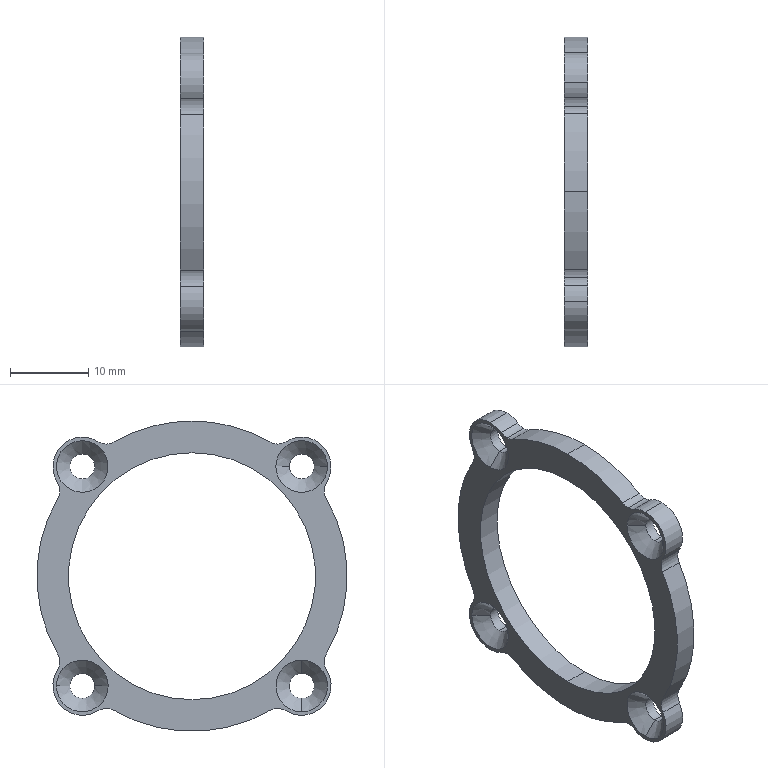Part | SolidWorks | features RefAxis 2, CirPattern 1, Extrusion 1, Fillet 1, RevCut 1 | 1 solid | 41 faces | box 3 x 39.6 x 39.6 mm | volume 1466 mm3 | cylinder 31 | cone 8 | plane 2 | commonest cylinder face diameters 4 x10 3.2 x8 7.5 x6 39.6 x5 31.5 x2
STEP:
#1=CARTESIAN_POINT('',(0.,10.93,16.862));
#2=VERTEX_POINT('',#1);
#3=CARTESIAN_POINT('',(0.,11.998,17.171));
#4=VERTEX_POINT('',#3);
#5=CARTESIAN_POINT('',(0.,10.93,18.862));
#6=DIRECTION('',(1.,0.,0.));
#7=DIRECTION('',(0.,0.,-1.));
#8=AXIS2_PLACEMENT_3D('',#5,#6,#7);
#9=CIRCLE('',#8,2.);
#10=EDGE_CURVE('',#2,#4,#9,.T.);
#11=ORIENTED_EDGE('',*,*,#10,.F.);
#12=CARTESIAN_POINT('',(3.,10.93,16.862));
#13=VERTEX_POINT('',#12);
#14=CARTESIAN_POINT('',(3.,10.93,16.862));
#15=DIRECTION('',(1.,0.,0.));
#16=VECTOR('',#15,1000.);
#17=LINE('',#14,#16);
#18=EDGE_CURVE('',#2,#13,#17,.T.);
#19=ORIENTED_EDGE('',*,*,#18,.T.);
#20=CARTESIAN_POINT('',(3.,11.998,17.171));
#21=VERTEX_POINT('',#20);
#22=CARTESIAN_POINT('',(3.,10.93,18.862));
#23=DIRECTION('',(-1.,0.,0.));
#24=DIRECTION('',(0.,0.,-1.));
#25=AXIS2_PLACEMENT_3D('',#22,#23,#24);
#26=CIRCLE('',#25,2.);
#27=EDGE_CURVE('',#21,#13,#26,.T.);
#28=ORIENTED_EDGE('',*,*,#27,.F.);
#29=CARTESIAN_POINT('',(3.,11.998,17.171));
#30=DIRECTION('',(1.,0.,0.));
#31=VECTOR('',#30,1000.);
#32=LINE('',#29,#31);
#33=EDGE_CURVE('',#4,#21,#32,.T.);
#34=ORIENTED_EDGE('',*,*,#33,.F.);
#35=EDGE_LOOP('',(#11,#19,#28,#34));
#36=FACE_OUTER_BOUND('',#35,.T.);
#37=CARTESIAN_POINT('',(3.,10.93,18.862));
#38=DIRECTION('',(1.,0.,0.));
#39=DIRECTION('',(0.,0.,-1.));
#40=AXIS2_PLACEMENT_3D('',#37,#38,#39);
#41=CYLINDRICAL_SURFACE('',#40,2.);
#42=ADVANCED_FACE('',(#36),#41,.F.);
#43=CARTESIAN_POINT('',(0.,-10.93,16.862));
#44=VERTEX_POINT('',#43);
#45=CARTESIAN_POINT('',(0.,-9.927,17.132));
#46=VERTEX_POINT('',#45);
#47=CARTESIAN_POINT('',(0.,-10.93,18.862));
#48=DIRECTION('',(1.,0.,0.));
#49=DIRECTION('',(0.,0.,-1.));
#50=AXIS2_PLACEMENT_3D('',#47,#48,#49);
#51=CIRCLE('',#50,2.);
#52=EDGE_CURVE('',#44,#46,#51,.T.);
#53=ORIENTED_EDGE('',*,*,#52,.F.);
#54=CARTESIAN_POINT('',(3.,-10.93,16.862));
#55=VERTEX_POINT('',#54);
#56=CARTESIAN_POINT('',(3.,-10.93,16.862));
#57=DIRECTION('',(1.,0.,0.));
#58=VECTOR('',#57,1000.);
#59=LINE('',#56,#58);
#60=EDGE_CURVE('',#44,#55,#59,.T.);
#61=ORIENTED_EDGE('',*,*,#60,.T.);
#62=CARTESIAN_POINT('',(3.,-9.927,17.132));
#63=VERTEX_POINT('',#62);
#64=CARTESIAN_POINT('',(3.,-10.93,18.862));
#65=DIRECTION('',(-1.,0.,0.));
#66=DIRECTION('',(0.,0.,-1.));
#67=AXIS2_PLACEMENT_3D('',#64,#65,#66);
#68=CIRCLE('',#67,2.);
#69=EDGE_CURVE('',#63,#55,#68,.T.);
#70=ORIENTED_EDGE('',*,*,#69,.F.);
#71=CARTESIAN_POINT('',(3.,-9.927,17.132));
#72=DIRECTION('',(1.,0.,0.));
#73=VECTOR('',#72,1000.);
#74=LINE('',#71,#73);
#75=EDGE_CURVE('',#46,#63,#74,.T.);
#76=ORIENTED_EDGE('',*,*,#75,.F.);
#77=EDGE_LOOP('',(#53,#61,#70,#76));
#78=FACE_OUTER_BOUND('',#77,.T.);
#79=CARTESIAN_POINT('',(3.,-10.93,18.862));
#80=DIRECTION('',(1.,0.,0.));
#81=DIRECTION('',(0.,0.,-1.));
#82=AXIS2_PLACEMENT_3D('',#79,#80,#81);
#83=CYLINDRICAL_SURFACE('',#82,2.);
#84=ADVANCED_FACE('',(#78),#83,.F.);
#85=CARTESIAN_POINT('',(1.7,14.001,-12.401));
#86=VERTEX_POINT('',#85);
#87=CARTESIAN_POINT('',(1.7,12.401,-14.001));
#88=VERTEX_POINT('',#87);
#89=CARTESIAN_POINT('',(1.7,14.001,-14.001));
#90=DIRECTION('',(1.,0.,0.));
#91=DIRECTION('',(0.,0.,1.));
#92=AXIS2_PLACEMENT_3D('',#89,#90,#91);
#93=CIRCLE('',#92,1.6);
#94=EDGE_CURVE('',#86,#88,#93,.T.);
#95=ORIENTED_EDGE('',*,*,#94,.T.);
#96=CARTESIAN_POINT('',(0.,10.701,-14.001));
#97=VERTEX_POINT('',#96);
#98=CARTESIAN_POINT('',(3.3,14.001,-14.001));
#99=DIRECTION('',(-0.7071,-0.7071,0.));
#100=VECTOR('',#99,1000.);
#101=LINE('',#98,#100);
#102=EDGE_CURVE('',#88,#97,#101,.T.);
#103=ORIENTED_EDGE('',*,*,#102,.T.);
#104=CARTESIAN_POINT('',(0.,17.301,-14.001));
#105=VERTEX_POINT('',#104);
#106=CARTESIAN_POINT('',(0.,14.001,-14.001));
#107=DIRECTION('',(1.,0.,0.));
#108=DIRECTION('',(0.,-1.,0.));
#109=AXIS2_PLACEMENT_3D('',#106,#107,#108);
#110=CIRCLE('',#109,3.3);
#111=EDGE_CURVE('',#105,#97,#110,.T.);
#112=ORIENTED_EDGE('',*,*,#111,.F.);
#113=CARTESIAN_POINT('',(1.7,15.601,-14.001));
#114=VERTEX_POINT('',#113);
#115=CARTESIAN_POINT('',(3.3,14.001,-14.001));
#116=DIRECTION('',(-0.7071,0.7071,0.));
#117=VECTOR('',#116,1000.);
#118=LINE('',#115,#117);
#119=EDGE_CURVE('',#114,#105,#118,.T.);
#120=ORIENTED_EDGE('',*,*,#119,.F.);
#121=CARTESIAN_POINT('',(1.7,14.001,-14.001));
#122=DIRECTION('',(1.,0.,0.));
#123=DIRECTION('',(0.,0.,1.));
#124=AXIS2_PLACEMENT_3D('',#121,#122,#123);
#125=CIRCLE('',#124,1.6);
#126=EDGE_CURVE('',#114,#86,#125,.T.);
#127=ORIENTED_EDGE('',*,*,#126,.T.);
#128=EDGE_LOOP('',(#95,#103,#112,#120,#127));
#129=FACE_OUTER_BOUND('',#128,.T.);
#130=CARTESIAN_POINT('',(-996.7,14.001,-14.001));
#131=DIRECTION('',(-1.,0.,0.));
#132=DIRECTION('',(0.,1.,0.));
#133=AXIS2_PLACEMENT_3D('',#130,#131,#132);
#134=CONICAL_SURFACE('',#133,1000.,0.7854);
#135=ADVANCED_FACE('',(#129),#134,.F.);
#136=CARTESIAN_POINT('',(1.7,-14.001,-15.601));
#137=VERTEX_POINT('',#136);
#138=CARTESIAN_POINT('',(1.7,-14.001,-12.401));
#139=VERTEX_POINT('',#138);
#140=CARTESIAN_POINT('',(1.7,-14.001,-14.001));
#141=DIRECTION('',(1.,0.,0.));
#142=DIRECTION('',(0.,0.,1.));
#143=AXIS2_PLACEMENT_3D('',#140,#141,#142);
#144=CIRCLE('',#143,1.6);
#145=EDGE_CURVE('',#137,#139,#144,.T.);
#146=ORIENTED_EDGE('',*,*,#145,.T.);
#147=CARTESIAN_POINT('',(0.,-14.001,-10.701));
#148=VERTEX_POINT('',#147);
#149=CARTESIAN_POINT('',(3.3,-14.001,-14.001));
#150=DIRECTION('',(-0.7071,0.,0.7071));
#151=VECTOR('',#150,1000.);
#152=LINE('',#149,#151);
#153=EDGE_CURVE('',#139,#148,#152,.T.);
#154=ORIENTED_EDGE('',*,*,#153,.T.);
#155=CARTESIAN_POINT('',(0.,-14.001,-17.301));
#156=VERTEX_POINT('',#155);
#157=CARTESIAN_POINT('',(0.,-14.001,-14.001));
#158=DIRECTION('',(1.,0.,0.));
#159=DIRECTION('',(0.,0.,1.));
#160=AXIS2_PLACEMENT_3D('',#157,#158,#159);
#161=CIRCLE('',#160,3.3);
#162=EDGE_CURVE('',#156,#148,#161,.T.);
#163=ORIENTED_EDGE('',*,*,#162,.F.);
#164=CARTESIAN_POINT('',(3.3,-14.001,-14.001));
#165=DIRECTION('',(-0.7071,0.,-0.7071));
#166=VECTOR('',#165,1000.);
#167=LINE('',#164,#166);
#168=EDGE_CURVE('',#137,#156,#167,.T.);
#169=ORIENTED_EDGE('',*,*,#168,.F.);
#170=EDGE_LOOP('',(#146,#154,#163,#169));
#171=FACE_OUTER_BOUND('',#170,.T.);
#172=CARTESIAN_POINT('',(-996.7,-14.001,-14.001));
#173=DIRECTION('',(-1.,0.,0.));
#174=DIRECTION('',(0.,0.,-1.));
#175=AXIS2_PLACEMENT_3D('',#172,#173,#174);
#176=CONICAL_SURFACE('',#175,1000.,0.7854);
#177=ADVANCED_FACE('',(#171),#176,.F.);
#178=CARTESIAN_POINT('',(1.7,-14.001,12.401));
#179=VERTEX_POINT('',#178);
#180=CARTESIAN_POINT('',(1.7,-12.401,14.001));
#181=VERTEX_POINT('',#180);
#182=CARTESIAN_POINT('',(1.7,-14.001,14.001));
#183=DIRECTION('',(1.,0.,0.));
#184=DIRECTION('',(0.,0.,1.));
#185=AXIS2_PLACEMENT_3D('',#182,#183,#184);
#186=CIRCLE('',#185,1.6);
#187=EDGE_CURVE('',#179,#181,#186,.T.);
#188=ORIENTED_EDGE('',*,*,#187,.T.);
#189=CARTESIAN_POINT('',(0.,-10.701,14.001));
#190=VERTEX_POINT('',#189);
#191=CARTESIAN_POINT('',(3.3,-14.001,14.001));
#192=DIRECTION('',(-0.7071,0.7071,0.));
#193=VECTOR('',#192,1000.);
#194=LINE('',#191,#193);
#195=EDGE_CURVE('',#181,#190,#194,.T.);
#196=ORIENTED_EDGE('',*,*,#195,.T.);
#197=CARTESIAN_POINT('',(0.,-17.301,14.001));
#198=VERTEX_POINT('',#197);
#199=CARTESIAN_POINT('',(0.,-14.001,14.001));
#200=DIRECTION('',(1.,0.,0.));
#201=DIRECTION('',(0.,1.,0.));
#202=AXIS2_PLACEMENT_3D('',#199,#200,#201);
#203=CIRCLE('',#202,3.3);
#204=EDGE_CURVE('',#198,#190,#203,.T.);
#205=ORIENTED_EDGE('',*,*,#204,.F.);
#206=CARTESIAN_POINT('',(1.7,-15.601,14.001));
#207=VERTEX_POINT('',#206);
#208=CARTESIAN_POINT('',(3.3,-14.001,14.001));
#209=DIRECTION('',(-0.7071,-0.7071,0.));
#210=VECTOR('',#209,1000.);
#211=LINE('',#208,#210);
#212=EDGE_CURVE('',#207,#198,#211,.T.);
#213=ORIENTED_EDGE('',*,*,#212,.F.);
#214=CARTESIAN_POINT('',(1.7,-14.001,14.001));
#215=DIRECTION('',(1.,0.,0.));
#216=DIRECTION('',(0.,0.,1.));
#217=AXIS2_PLACEMENT_3D('',#214,#215,#216);
#218=CIRCLE('',#217,1.6);
#219=EDGE_CURVE('',#207,#179,#218,.T.);
#220=ORIENTED_EDGE('',*,*,#219,.T.);
#221=EDGE_LOOP('',(#188,#196,#205,#213,#220));
#222=FACE_OUTER_BOUND('',#221,.T.);
#223=CARTESIAN_POINT('',(-996.7,-14.001,14.001));
#224=DIRECTION('',(-1.,0.,0.));
#225=DIRECTION('',(0.,-1.,0.));
#226=AXIS2_PLACEMENT_3D('',#223,#224,#225);
#227=CONICAL_SURFACE('',#226,1000.,0.7854);
#228=ADVANCED_FACE('',(#222),#227,.F.);
#229=CARTESIAN_POINT('',(1.7,14.001,15.601));
#230=VERTEX_POINT('',#229);
#231=CARTESIAN_POINT('',(1.7,14.001,12.401));
#232=VERTEX_POINT('',#231);
#233=CARTESIAN_POINT('',(1.7,14.001,14.001));
#234=DIRECTION('',(1.,0.,0.));
#235=DIRECTION('',(0.,0.,1.));
#236=AXIS2_PLACEMENT_3D('',#233,#234,#235);
#237=CIRCLE('',#236,1.6);
#238=EDGE_CURVE('',#230,#232,#237,.T.);
#239=ORIENTED_EDGE('',*,*,#238,.T.);
#240=CARTESIAN_POINT('',(0.,14.001,10.701));
#241=VERTEX_POINT('',#240);
#242=CARTESIAN_POINT('',(3.3,14.001,14.001));
#243=DIRECTION('',(-0.7071,0.,-0.7071));
#244=VECTOR('',#243,1000.);
#245=LINE('',#242,#244);
#246=EDGE_CURVE('',#232,#241,#245,.T.);
#247=ORIENTED_EDGE('',*,*,#246,.T.);
#248=CARTESIAN_POINT('',(0.,14.001,17.301));
#249=VERTEX_POINT('',#248);
#250=CARTESIAN_POINT('',(0.,14.001,14.001));
#251=DIRECTION('',(1.,0.,0.));
#252=DIRECTION('',(0.,0.,-1.));
#253=AXIS2_PLACEMENT_3D('',#250,#251,#252);
#254=CIRCLE('',#253,3.3);
#255=EDGE_CURVE('',#249,#241,#254,.T.);
#256=ORIENTED_EDGE('',*,*,#255,.F.);
#257=CARTESIAN_POINT('',(3.3,14.001,14.001));
#258=DIRECTION('',(-0.7071,0.,0.7071));
#259=VECTOR('',#258,1000.);
#260=LINE('',#257,#259);
#261=EDGE_CURVE('',#230,#249,#260,.T.);
#262=ORIENTED_EDGE('',*,*,#261,.F.);
#263=EDGE_LOOP('',(#239,#247,#256,#262));
#264=FACE_OUTER_BOUND('',#263,.T.);
#265=CARTESIAN_POINT('',(-996.7,14.001,14.001));
#266=DIRECTION('',(-1.,0.,0.));
#267=DIRECTION('',(0.,0.,1.));
#268=AXIS2_PLACEMENT_3D('',#265,#266,#267);
#269=CONICAL_SURFACE('',#268,1000.,0.7854);
#270=ADVANCED_FACE('',(#264),#269,.F.);
#271=CARTESIAN_POINT('',(3.,14.001,-12.401));
#272=VERTEX_POINT('',#271);
#273=CARTESIAN_POINT('',(3.,14.001,-15.601));
#274=VERTEX_POINT('',#273);
#275=CARTESIAN_POINT('',(3.,14.001,-14.001));
#276=DIRECTION('',(1.,0.,0.));
#277=DIRECTION('',(0.,0.,-1.));
#278=AXIS2_PLACEMENT_3D('',#275,#276,#277);
#279=CIRCLE('',#278,1.6);
#280=EDGE_CURVE('',#272,#274,#279,.T.);
#281=ORIENTED_EDGE('',*,*,#280,.T.);
#282=CARTESIAN_POINT('',(1.7,14.001,-15.601));
#283=VERTEX_POINT('',#282);
#284=CARTESIAN_POINT('',(3.,14.001,-15.601));
#285=DIRECTION('',(-1.,0.,0.));
#286=VECTOR('',#285,1000.);
#287=LINE('',#284,#286);
#288=EDGE_CURVE('',#274,#283,#287,.T.);
#289=ORIENTED_EDGE('',*,*,#288,.T.);
#290=CARTESIAN_POINT('',(1.7,14.001,-14.001));
#291=DIRECTION('',(1.,0.,0.));
#292=DIRECTION('',(0.,0.,1.));
#293=AXIS2_PLACEMENT_3D('',#290,#291,#292);
#294=CIRCLE('',#293,1.6);
#295=EDGE_CURVE('',#88,#283,#294,.T.);
#296=ORIENTED_EDGE('',*,*,#295,.F.);
#297=ORIENTED_EDGE('',*,*,#94,.F.);
#298=CARTESIAN_POINT('',(3.,14.001,-12.401));
#299=DIRECTION('',(-1.,0.,0.));
#300=VECTOR('',#299,1000.);
#301=LINE('',#298,#300);
#302=EDGE_CURVE('',#272,#86,#301,.T.);
#303=ORIENTED_EDGE('',*,*,#302,.F.);
#304=EDGE_LOOP('',(#281,#289,#296,#297,#303));
#305=FACE_OUTER_BOUND('',#304,.T.);
#306=CARTESIAN_POINT('',(3.,14.001,-14.001));
#307=DIRECTION('',(-1.,0.,0.));
#308=DIRECTION('',(0.,0.,1.));
#309=AXIS2_PLACEMENT_3D('',#306,#307,#308);
#310=CYLINDRICAL_SURFACE('',#309,1.6);
#311=ADVANCED_FACE('',(#305),#310,.F.);
#312=CARTESIAN_POINT('',(3.,14.001,15.601));
#313=VERTEX_POINT('',#312);
#314=CARTESIAN_POINT('',(3.,14.001,12.401));
#315=VERTEX_POINT('',#314);
#316=CARTESIAN_POINT('',(3.,14.001,14.001));
#317=DIRECTION('',(1.,0.,0.));
#318=DIRECTION('',(0.,0.,-1.));
#319=AXIS2_PLACEMENT_3D('',#316,#317,#318);
#320=CIRCLE('',#319,1.6);
#321=EDGE_CURVE('',#313,#315,#320,.T.);
#322=ORIENTED_EDGE('',*,*,#321,.T.);
#323=CARTESIAN_POINT('',(3.,14.001,12.401));
#324=DIRECTION('',(-1.,0.,0.));
#325=VECTOR('',#324,1000.);
#326=LINE('',#323,#325);
#327=EDGE_CURVE('',#315,#232,#326,.T.);
#328=ORIENTED_EDGE('',*,*,#327,.T.);
#329=ORIENTED_EDGE('',*,*,#238,.F.);
#330=CARTESIAN_POINT('',(3.,14.001,15.601));
#331=DIRECTION('',(-1.,0.,0.));
#332=VECTOR('',#331,1000.);
#333=LINE('',#330,#332);
#334=EDGE_CURVE('',#313,#230,#333,.T.);
#335=ORIENTED_EDGE('',*,*,#334,.F.);
#336=EDGE_LOOP('',(#322,#328,#329,#335));
#337=FACE_OUTER_BOUND('',#336,.T.);
#338=CARTESIAN_POINT('',(3.,14.001,14.001));
#339=DIRECTION('',(-1.,0.,0.));
#340=DIRECTION('',(0.,0.,1.));
#341=AXIS2_PLACEMENT_3D('',#338,#339,#340);
#342=CYLINDRICAL_SURFACE('',#341,1.6);
#343=ADVANCED_FACE('',(#337),#342,.F.);
#344=CARTESIAN_POINT('',(3.,-14.001,15.601));
#345=VERTEX_POINT('',#344);
#346=CARTESIAN_POINT('',(3.,-14.001,12.401));
#347=VERTEX_POINT('',#346);
#348=CARTESIAN_POINT('',(3.,-14.001,14.001));
#349=DIRECTION('',(1.,0.,0.));
#350=DIRECTION('',(0.,0.,-1.));
#351=AXIS2_PLACEMENT_3D('',#348,#349,#350);
#352=CIRCLE('',#351,1.6);
#353=EDGE_CURVE('',#345,#347,#352,.T.);
#354=ORIENTED_EDGE('',*,*,#353,.T.);
#355=CARTESIAN_POINT('',(3.,-14.001,12.401));
#356=DIRECTION('',(-1.,0.,0.));
#357=VECTOR('',#356,1000.);
#358=LINE('',#355,#357);
#359=EDGE_CURVE('',#347,#179,#358,.T.);
#360=ORIENTED_EDGE('',*,*,#359,.T.);
#361=ORIENTED_EDGE('',*,*,#219,.F.);
#362=CARTESIAN_POINT('',(1.7,-14.001,15.601));
#363=VERTEX_POINT('',#362);
#364=CARTESIAN_POINT('',(1.7,-14.001,14.001));
#365=DIRECTION('',(1.,0.,0.));
#366=DIRECTION('',(0.,0.,1.));
#367=AXIS2_PLACEMENT_3D('',#364,#365,#366);
#368=CIRCLE('',#367,1.6);
#369=EDGE_CURVE('',#363,#207,#368,.T.);
#370=ORIENTED_EDGE('',*,*,#369,.F.);
#371=CARTESIAN_POINT('',(3.,-14.001,15.601));
#372=DIRECTION('',(-1.,0.,0.));
#373=VECTOR('',#372,1000.);
#374=LINE('',#371,#373);
#375=EDGE_CURVE('',#345,#363,#374,.T.);
#376=ORIENTED_EDGE('',*,*,#375,.F.);
#377=EDGE_LOOP('',(#354,#360,#361,#370,#376));
#378=FACE_OUTER_BOUND('',#377,.T.);
#379=CARTESIAN_POINT('',(3.,-14.001,14.001));
#380=DIRECTION('',(-1.,0.,0.));
#381=DIRECTION('',(0.,0.,1.));
#382=AXIS2_PLACEMENT_3D('',#379,#380,#381);
#383=CYLINDRICAL_SURFACE('',#382,1.6);
#384=ADVANCED_FACE('',(#378),#383,.F.);
#385=CARTESIAN_POINT('',(3.,-14.001,-12.401));
#386=VERTEX_POINT('',#385);
#387=CARTESIAN_POINT('',(3.,-14.001,-15.601));
#388=VERTEX_POINT('',#387);
#389=CARTESIAN_POINT('',(3.,-14.001,-14.001));
#390=DIRECTION('',(1.,0.,0.));
#391=DIRECTION('',(0.,0.,-1.));
#392=AXIS2_PLACEMENT_3D('',#389,#390,#391);
#393=CIRCLE('',#392,1.6);
#394=EDGE_CURVE('',#386,#388,#393,.T.);
#395=ORIENTED_EDGE('',*,*,#394,.T.);
#396=CARTESIAN_POINT('',(3.,-14.001,-15.601));
#397=DIRECTION('',(-1.,0.,0.));
#398=VECTOR('',#397,1000.);
#399=LINE('',#396,#398);
#400=EDGE_CURVE('',#388,#137,#399,.T.);
#401=ORIENTED_EDGE('',*,*,#400,.T.);
#402=CARTESIAN_POINT('',(1.7,-14.001,-14.001));
#403=DIRECTION('',(1.,0.,0.));
#404=DIRECTION('',(0.,0.,1.));
#405=AXIS2_PLACEMENT_3D('',#402,#403,#404);
#406=CIRCLE('',#405,1.6);
#407=EDGE_CURVE('',#139,#137,#406,.T.);
#408=ORIENTED_EDGE('',*,*,#407,.F.);
#409=CARTESIAN_POINT('',(3.,-14.001,-12.401));
#410=DIRECTION('',(-1.,0.,0.));
#411=VECTOR('',#410,1000.);
#412=LINE('',#409,#411);
#413=EDGE_CURVE('',#386,#139,#412,.T.);
#414=ORIENTED_EDGE('',*,*,#413,.F.);
#415=EDGE_LOOP('',(#395,#401,#408,#414));
#416=FACE_OUTER_BOUND('',#415,.T.);
#417=CARTESIAN_POINT('',(3.,-14.001,-14.001));
#418=DIRECTION('',(-1.,0.,0.));
#419=DIRECTION('',(0.,0.,1.));
#420=AXIS2_PLACEMENT_3D('',#417,#418,#419);
#421=CYLINDRICAL_SURFACE('',#420,1.6);
#422=ADVANCED_FACE('',(#416),#421,.F.);
#423=CARTESIAN_POINT('',(3.,0.,15.75));
#424=VERTEX_POINT('',#423);
#425=CARTESIAN_POINT('',(3.,0.,-15.75));
#426=VERTEX_POINT('',#425);
#427=CARTESIAN_POINT('',(3.,0.,0.));
#428=DIRECTION('',(1.,0.,0.));
#429=DIRECTION('',(0.,0.,-1.));
#430=AXIS2_PLACEMENT_3D('',#427,#428,#429);
#431=CIRCLE('',#430,15.75);
#432=EDGE_CURVE('',#424,#426,#431,.T.);
#433=ORIENTED_EDGE('',*,*,#432,.T.);
#434=CARTESIAN_POINT('',(0.,0.,-15.75));
#435=VERTEX_POINT('',#434);
#436=CARTESIAN_POINT('',(3.,0.,-15.75));
#437=DIRECTION('',(-1.,0.,0.));
#438=VECTOR('',#437,1000.);
#439=LINE('',#436,#438);
#440=EDGE_CURVE('',#426,#435,#439,.T.);
#441=ORIENTED_EDGE('',*,*,#440,.T.);
#442=CARTESIAN_POINT('',(0.,0.,15.75));
#443=VERTEX_POINT('',#442);
#444=CARTESIAN_POINT('',(0.,0.,0.));
#445=DIRECTION('',(1.,0.,0.));
#446=DIRECTION('',(0.,0.,-1.));
#447=AXIS2_PLACEMENT_3D('',#444,#445,#446);
#448=CIRCLE('',#447,15.75);
#449=EDGE_CURVE('',#443,#435,#448,.T.);
#450=ORIENTED_EDGE('',*,*,#449,.F.);
#451=CARTESIAN_POINT('',(3.,0.,15.75));
#452=DIRECTION('',(-1.,0.,0.));
#453=VECTOR('',#452,1000.);
#454=LINE('',#451,#453);
#455=EDGE_CURVE('',#424,#443,#454,.T.);
#456=ORIENTED_EDGE('',*,*,#455,.F.);
#457=EDGE_LOOP('',(#433,#441,#450,#456));
#458=FACE_OUTER_BOUND('',#457,.T.);
#459=CARTESIAN_POINT('',(3.,0.,0.));
#460=DIRECTION('',(-1.,0.,0.));
#461=DIRECTION('',(0.,0.,1.));
#462=AXIS2_PLACEMENT_3D('',#459,#460,#461);
#463=CYLINDRICAL_SURFACE('',#462,15.75);
#464=ADVANCED_FACE('',(#458),#463,.F.);
#465=CARTESIAN_POINT('',(3.,-14.001,17.751));
#466=VERTEX_POINT('',#465);
#467=CARTESIAN_POINT('',(3.,-17.171,11.998));
#468=VERTEX_POINT('',#467);
#469=CARTESIAN_POINT('',(3.,-14.001,14.001));
#470=DIRECTION('',(1.,0.,0.));
#471=DIRECTION('',(0.,0.,-1.));
#472=AXIS2_PLACEMENT_3D('',#469,#470,#471);
#473=CIRCLE('',#472,3.75);
#474=EDGE_CURVE('',#466,#468,#473,.T.);
#475=ORIENTED_EDGE('',*,*,#474,.F.);
#476=CARTESIAN_POINT('',(0.,-14.001,17.751));
#477=VERTEX_POINT('',#476);
#478=CARTESIAN_POINT('',(3.,-14.001,17.751));
#479=DIRECTION('',(-1.,0.,0.));
#480=VECTOR('',#479,1000.);
#481=LINE('',#478,#480);
#482=EDGE_CURVE('',#466,#477,#481,.T.);
#483=ORIENTED_EDGE('',*,*,#482,.T.);
#484=CARTESIAN_POINT('',(0.,-17.171,11.998));
#485=VERTEX_POINT('',#484);
#486=CARTESIAN_POINT('',(0.,-14.001,14.001));
#487=DIRECTION('',(1.,0.,0.));
#488=DIRECTION('',(0.,0.,-1.));
#489=AXIS2_PLACEMENT_3D('',#486,#487,#488);
#490=CIRCLE('',#489,3.75);
#491=EDGE_CURVE('',#477,#485,#490,.T.);
#492=ORIENTED_EDGE('',*,*,#491,.T.);
#493=CARTESIAN_POINT('',(3.,-17.171,11.998));
#494=DIRECTION('',(1.,0.,0.));
#495=VECTOR('',#494,1000.);
#496=LINE('',#493,#495);
#497=EDGE_CURVE('',#485,#468,#496,.T.);
#498=ORIENTED_EDGE('',*,*,#497,.T.);
#499=EDGE_LOOP('',(#475,#483,#492,#498));
#500=FACE_OUTER_BOUND('',#499,.T.);
#501=CARTESIAN_POINT('',(3.,-14.001,14.001));
#502=DIRECTION('',(-1.,0.,0.));
#503=DIRECTION('',(0.,0.,1.));
#504=AXIS2_PLACEMENT_3D('',#501,#502,#503);
#505=CYLINDRICAL_SURFACE('',#504,3.75);
#506=ADVANCED_FACE('',(#500),#505,.T.);
#507=CARTESIAN_POINT('',(3.,0.,19.8));
#508=VERTEX_POINT('',#507);
#509=CARTESIAN_POINT('',(3.,0.,0.));
#510=DIRECTION('',(1.,0.,0.));
#511=DIRECTION('',(0.,0.,-1.));
#512=AXIS2_PLACEMENT_3D('',#509,#510,#511);
#513=CIRCLE('',#512,19.8);
#514=EDGE_CURVE('',#508,#63,#513,.T.);
#515=ORIENTED_EDGE('',*,*,#514,.F.);
#516=CARTESIAN_POINT('',(0.,0.,19.8));
#517=VERTEX_POINT('',#516);
#518=CARTESIAN_POINT('',(3.,0.,19.8));
#519=DIRECTION('',(-1.,0.,0.));
#520=VECTOR('',#519,1000.);
#521=LINE('',#518,#520);
#522=EDGE_CURVE('',#508,#517,#521,.T.);
#523=ORIENTED_EDGE('',*,*,#522,.T.);
#524=CARTESIAN_POINT('',(0.,0.,0.));
#525=DIRECTION('',(1.,0.,0.));
#526=DIRECTION('',(0.,0.,-1.));
#527=AXIS2_PLACEMENT_3D('',#524,#525,#526);
#528=CIRCLE('',#527,19.8);
#529=EDGE_CURVE('',#517,#46,#528,.T.);
#530=ORIENTED_EDGE('',*,*,#529,.T.);
#531=ORIENTED_EDGE('',*,*,#75,.T.);
#532=EDGE_LOOP('',(#515,#523,#530,#531));
#533=FACE_OUTER_BOUND('',#532,.T.);
#534=CARTESIAN_POINT('',(3.,0.,0.));
#535=DIRECTION('',(-1.,0.,0.));
#536=DIRECTION('',(0.,0.,1.));
#537=AXIS2_PLACEMENT_3D('',#534,#535,#536);
#538=CYLINDRICAL_SURFACE('',#537,19.8);
#539=ADVANCED_FACE('',(#533),#538,.T.);
#540=CARTESIAN_POINT('',(3.,14.001,17.751));
#541=VERTEX_POINT('',#540);
#542=CARTESIAN_POINT('',(3.,14.001,14.001));
#543=DIRECTION('',(1.,0.,0.));
#544=DIRECTION('',(0.,0.,-1.));
#545=AXIS2_PLACEMENT_3D('',#542,#543,#544);
#546=CIRCLE('',#545,3.75);
#547=EDGE_CURVE('',#541,#21,#546,.T.);
#548=ORIENTED_EDGE('',*,*,#547,.F.);
#549=CARTESIAN_POINT('',(0.,14.001,17.751));
#550=VERTEX_POINT('',#549);
#551=CARTESIAN_POINT('',(3.,14.001,17.751));
#552=DIRECTION('',(-1.,0.,0.));
#553=VECTOR('',#552,1000.);
#554=LINE('',#551,#553);
#555=EDGE_CURVE('',#541,#550,#554,.T.);
#556=ORIENTED_EDGE('',*,*,#555,.T.);
#557=CARTESIAN_POINT('',(0.,14.001,14.001));
#558=DIRECTION('',(1.,0.,0.));
#559=DIRECTION('',(0.,0.,-1.));
#560=AXIS2_PLACEMENT_3D('',#557,#558,#559);
#561=CIRCLE('',#560,3.75);
#562=EDGE_CURVE('',#550,#4,#561,.T.);
#563=ORIENTED_EDGE('',*,*,#562,.T.);
#564=ORIENTED_EDGE('',*,*,#33,.T.);
#565=EDGE_LOOP('',(#548,#556,#563,#564));
#566=FACE_OUTER_BOUND('',#565,.T.);
#567=CARTESIAN_POINT('',(3.,14.001,14.001));
#568=DIRECTION('',(-1.,0.,0.));
#569=DIRECTION('',(0.,0.,1.));
#570=AXIS2_PLACEMENT_3D('',#567,#568,#569);
#571=CYLINDRICAL_SURFACE('',#570,3.75);
#572=ADVANCED_FACE('',(#566),#571,.T.);
#573=ORIENTED_EDGE('',*,*,#321,.F.);
#574=CARTESIAN_POINT('',(3.,14.001,14.001));
#575=DIRECTION('',(1.,0.,0.));
#576=DIRECTION('',(0.,0.,-1.));
#577=AXIS2_PLACEMENT_3D('',#574,#575,#576);
#578=CIRCLE('',#577,1.6);
#579=EDGE_CURVE('',#315,#313,#578,.T.);
#580=ORIENTED_EDGE('',*,*,#579,.F.);
#581=EDGE_LOOP('',(#573,#580));
#582=FACE_BOUND('',#581,.T.);
#583=ORIENTED_EDGE('',*,*,#394,.F.);
#584=CARTESIAN_POINT('',(3.,-14.001,-14.001));
#585=DIRECTION('',(1.,0.,0.));
#586=DIRECTION('',(0.,0.,-1.));
#587=AXIS2_PLACEMENT_3D('',#584,#585,#586);
#588=CIRCLE('',#587,1.6);
#589=EDGE_CURVE('',#388,#386,#588,.T.);
#590=ORIENTED_EDGE('',*,*,#589,.F.);
#591=EDGE_LOOP('',(#583,#590));
#592=FACE_BOUND('',#591,.T.);
#593=CARTESIAN_POINT('',(3.,-17.171,-11.998));
#594=VERTEX_POINT('',#593);
#595=CARTESIAN_POINT('',(3.,-11.998,-17.171));
#596=VERTEX_POINT('',#595);
#597=CARTESIAN_POINT('',(3.,-14.001,-14.001));
#598=DIRECTION('',(1.,0.,0.));
#599=DIRECTION('',(0.,0.,-1.));
#600=AXIS2_PLACEMENT_3D('',#597,#598,#599);
#601=CIRCLE('',#600,3.75);
#602=EDGE_CURVE('',#594,#596,#601,.T.);
#603=ORIENTED_EDGE('',*,*,#602,.T.);
#604=CARTESIAN_POINT('',(3.,-9.927,-17.132));
#605=VERTEX_POINT('',#604);
#606=CARTESIAN_POINT('',(3.,-10.93,-18.862));
#607=DIRECTION('',(-1.,0.,0.));
#608=DIRECTION('',(0.,0.,-1.));
#609=AXIS2_PLACEMENT_3D('',#606,#607,#608);
#610=CIRCLE('',#609,2.);
#611=EDGE_CURVE('',#596,#605,#610,.T.);
#612=ORIENTED_EDGE('',*,*,#611,.T.);
#613=CARTESIAN_POINT('',(3.,9.927,-17.132));
#614=VERTEX_POINT('',#613);
#615=CARTESIAN_POINT('',(3.,0.,0.));
#616=DIRECTION('',(1.,0.,0.));
#617=DIRECTION('',(0.,0.,-1.));
#618=AXIS2_PLACEMENT_3D('',#615,#616,#617);
#619=CIRCLE('',#618,19.8);
#620=EDGE_CURVE('',#605,#614,#619,.T.);
#621=ORIENTED_EDGE('',*,*,#620,.T.);
#622=CARTESIAN_POINT('',(3.,11.998,-17.171));
#623=VERTEX_POINT('',#622);
#624=CARTESIAN_POINT('',(3.,10.93,-18.862));
#625=DIRECTION('',(-1.,0.,0.));
#626=DIRECTION('',(0.,0.,-1.));
#627=AXIS2_PLACEMENT_3D('',#624,#625,#626);
#628=CIRCLE('',#627,2.);
#629=EDGE_CURVE('',#614,#623,#628,.T.);
#630=ORIENTED_EDGE('',*,*,#629,.T.);
#631=CARTESIAN_POINT('',(3.,17.171,-11.998));
#632=VERTEX_POINT('',#631);
#633=CARTESIAN_POINT('',(3.,14.001,-14.001));
#634=DIRECTION('',(1.,0.,0.));
#635=DIRECTION('',(0.,0.,-1.));
#636=AXIS2_PLACEMENT_3D('',#633,#634,#635);
#637=CIRCLE('',#636,3.75);
#638=EDGE_CURVE('',#623,#632,#637,.T.);
#639=ORIENTED_EDGE('',*,*,#638,.T.);
#640=CARTESIAN_POINT('',(3.,17.132,-9.927));
#641=VERTEX_POINT('',#640);
#642=CARTESIAN_POINT('',(3.,18.862,-10.93));
#643=DIRECTION('',(-1.,0.,0.));
#644=DIRECTION('',(0.,0.,-1.));
#645=AXIS2_PLACEMENT_3D('',#642,#643,#644);
#646=CIRCLE('',#645,2.);
#647=EDGE_CURVE('',#632,#641,#646,.T.);
#648=ORIENTED_EDGE('',*,*,#647,.T.);
#649=CARTESIAN_POINT('',(3.,17.132,9.927));
#650=VERTEX_POINT('',#649);
#651=CARTESIAN_POINT('',(3.,0.,0.));
#652=DIRECTION('',(1.,0.,0.));
#653=DIRECTION('',(0.,0.,-1.));
#654=AXIS2_PLACEMENT_3D('',#651,#652,#653);
#655=CIRCLE('',#654,19.8);
#656=EDGE_CURVE('',#641,#650,#655,.T.);
#657=ORIENTED_EDGE('',*,*,#656,.T.);
#658=CARTESIAN_POINT('',(3.,17.171,11.998));
#659=VERTEX_POINT('',#658);
#660=CARTESIAN_POINT('',(3.,18.862,10.93));
#661=DIRECTION('',(-1.,0.,0.));
#662=DIRECTION('',(0.,0.,-1.));
#663=AXIS2_PLACEMENT_3D('',#660,#661,#662);
#664=CIRCLE('',#663,2.);
#665=EDGE_CURVE('',#650,#659,#664,.T.);
#666=ORIENTED_EDGE('',*,*,#665,.T.);
#667=CARTESIAN_POINT('',(3.,14.001,14.001));
#668=DIRECTION('',(1.,0.,0.));
#669=DIRECTION('',(0.,0.,-1.));
#670=AXIS2_PLACEMENT_3D('',#667,#668,#669);
#671=CIRCLE('',#670,3.75);
#672=EDGE_CURVE('',#659,#541,#671,.T.);
#673=ORIENTED_EDGE('',*,*,#672,.T.);
#674=ORIENTED_EDGE('',*,*,#547,.T.);
#675=ORIENTED_EDGE('',*,*,#27,.T.);
#676=CARTESIAN_POINT('',(3.,9.927,17.132));
#677=VERTEX_POINT('',#676);
#678=CARTESIAN_POINT('',(3.,10.93,18.862));
#679=DIRECTION('',(-1.,0.,0.));
#680=DIRECTION('',(0.,0.,-1.));
#681=AXIS2_PLACEMENT_3D('',#678,#679,#680);
#682=CIRCLE('',#681,2.);
#683=EDGE_CURVE('',#13,#677,#682,.T.);
#684=ORIENTED_EDGE('',*,*,#683,.T.);
#685=CARTESIAN_POINT('',(3.,0.,0.));
#686=DIRECTION('',(1.,0.,0.));
#687=DIRECTION('',(0.,0.,-1.));
#688=AXIS2_PLACEMENT_3D('',#685,#686,#687);
#689=CIRCLE('',#688,19.8);
#690=EDGE_CURVE('',#677,#508,#689,.T.);
#691=ORIENTED_EDGE('',*,*,#690,.T.);
#692=ORIENTED_EDGE('',*,*,#514,.T.);
#693=ORIENTED_EDGE('',*,*,#69,.T.);
#694=CARTESIAN_POINT('',(3.,-11.998,17.171));
#695=VERTEX_POINT('',#694);
#696=CARTESIAN_POINT('',(3.,-10.93,18.862));
#697=DIRECTION('',(-1.,0.,0.));
#698=DIRECTION('',(0.,0.,-1.));
#699=AXIS2_PLACEMENT_3D('',#696,#697,#698);
#700=CIRCLE('',#699,2.);
#701=EDGE_CURVE('',#55,#695,#700,.T.);
#702=ORIENTED_EDGE('',*,*,#701,.T.);
#703=CARTESIAN_POINT('',(3.,-14.001,14.001));
#704=DIRECTION('',(1.,0.,0.));
#705=DIRECTION('',(0.,0.,-1.));
#706=AXIS2_PLACEMENT_3D('',#703,#704,#705);
#707=CIRCLE('',#706,3.75);
#708=EDGE_CURVE('',#695,#466,#707,.T.);
#709=ORIENTED_EDGE('',*,*,#708,.T.);
#710=ORIENTED_EDGE('',*,*,#474,.T.);
#711=CARTESIAN_POINT('',(3.,-17.132,9.927));
#712=VERTEX_POINT('',#711);
#713=CARTESIAN_POINT('',(3.,-18.862,10.93));
#714=DIRECTION('',(-1.,0.,0.));
#715=DIRECTION('',(0.,0.,-1.));
#716=AXIS2_PLACEMENT_3D('',#713,#714,#715);
#717=CIRCLE('',#716,2.);
#718=EDGE_CURVE('',#468,#712,#717,.T.);
#719=ORIENTED_EDGE('',*,*,#718,.T.);
#720=CARTESIAN_POINT('',(3.,-17.132,-9.927));
#721=VERTEX_POINT('',#720);
#722=CARTESIAN_POINT('',(3.,0.,0.));
#723=DIRECTION('',(1.,0.,0.));
#724=DIRECTION('',(0.,0.,-1.));
#725=AXIS2_PLACEMENT_3D('',#722,#723,#724);
#726=CIRCLE('',#725,19.8);
#727=EDGE_CURVE('',#712,#721,#726,.T.);
#728=ORIENTED_EDGE('',*,*,#727,.T.);
#729=CARTESIAN_POINT('',(3.,-18.862,-10.93));
#730=DIRECTION('',(-1.,0.,0.));
#731=DIRECTION('',(0.,0.,-1.));
#732=AXIS2_PLACEMENT_3D('',#729,#730,#731);
#733=CIRCLE('',#732,2.);
#734=EDGE_CURVE('',#721,#594,#733,.T.);
#735=ORIENTED_EDGE('',*,*,#734,.T.);
#736=EDGE_LOOP('',(#603,#612,#621,#630,#639,#648,#657,#666,#673,#674,#675,#684,#691,#692,#693,#702,#709,#710,#719,#728,#735));
#737=FACE_OUTER_BOUND('',#736,.T.);
#738=ORIENTED_EDGE('',*,*,#432,.F.);
#739=CARTESIAN_POINT('',(3.,0.,0.));
#740=DIRECTION('',(1.,0.,0.));
#741=DIRECTION('',(0.,0.,-1.));
#742=AXIS2_PLACEMENT_3D('',#739,#740,#741);
#743=CIRCLE('',#742,15.75);
#744=EDGE_CURVE('',#426,#424,#743,.T.);
#745=ORIENTED_EDGE('',*,*,#744,.F.);
#746=EDGE_LOOP('',(#738,#745));
#747=FACE_BOUND('',#746,.T.);
#748=ORIENTED_EDGE('',*,*,#353,.F.);
#749=CARTESIAN_POINT('',(3.,-14.001,14.001));
#750=DIRECTION('',(1.,0.,0.));
#751=DIRECTION('',(0.,0.,-1.));
#752=AXIS2_PLACEMENT_3D('',#749,#750,#751);
#753=CIRCLE('',#752,1.6);
#754=EDGE_CURVE('',#347,#345,#753,.T.);
#755=ORIENTED_EDGE('',*,*,#754,.F.);
#756=EDGE_LOOP('',(#748,#755));
#757=FACE_BOUND('',#756,.T.);
#758=ORIENTED_EDGE('',*,*,#280,.F.);
#759=CARTESIAN_POINT('',(3.,14.001,-14.001));
#760=DIRECTION('',(1.,0.,0.));
#761=DIRECTION('',(0.,0.,-1.));
#762=AXIS2_PLACEMENT_3D('',#759,#760,#761);
#763=CIRCLE('',#762,1.6);
#764=EDGE_CURVE('',#274,#272,#763,.T.);
#765=ORIENTED_EDGE('',*,*,#764,.F.);
#766=EDGE_LOOP('',(#758,#765));
#767=FACE_BOUND('',#766,.T.);
#768=CARTESIAN_POINT('',(3.,7.,-7.));
#769=DIRECTION('',(1.,0.,0.));
#770=DIRECTION('',(0.,0.,-1.));
#771=AXIS2_PLACEMENT_3D('',#768,#769,#770);
#772=PLANE('',#771);
#773=ADVANCED_FACE('',(#582,#592,#737,#747,#757,#767),#772,.T.);
#774=ORIENTED_EDGE('',*,*,#111,.T.);
#775=CARTESIAN_POINT('',(0.,14.001,-14.001));
#776=DIRECTION('',(1.,0.,0.));
#777=DIRECTION('',(0.,-1.,0.));
#778=AXIS2_PLACEMENT_3D('',#775,#776,#777);
#779=CIRCLE('',#778,3.3);
#780=EDGE_CURVE('',#97,#105,#779,.T.);
#781=ORIENTED_EDGE('',*,*,#780,.T.);
#782=EDGE_LOOP('',(#774,#781));
#783=FACE_BOUND('',#782,.T.);
#784=ORIENTED_EDGE('',*,*,#162,.T.);
#785=CARTESIAN_POINT('',(0.,-14.001,-14.001));
#786=DIRECTION('',(1.,0.,0.));
#787=DIRECTION('',(0.,0.,1.));
#788=AXIS2_PLACEMENT_3D('',#785,#786,#787);
#789=CIRCLE('',#788,3.3);
#790=EDGE_CURVE('',#148,#156,#789,.T.);
#791=ORIENTED_EDGE('',*,*,#790,.T.);
#792=EDGE_LOOP('',(#784,#791));
#793=FACE_BOUND('',#792,.T.);
#794=ORIENTED_EDGE('',*,*,#204,.T.);
#795=CARTESIAN_POINT('',(0.,-14.001,14.001));
#796=DIRECTION('',(1.,0.,0.));
#797=DIRECTION('',(0.,1.,0.));
#798=AXIS2_PLACEMENT_3D('',#795,#796,#797);
#799=CIRCLE('',#798,3.3);
#800=EDGE_CURVE('',#190,#198,#799,.T.);
#801=ORIENTED_EDGE('',*,*,#800,.T.);
#802=EDGE_LOOP('',(#794,#801));
#803=FACE_BOUND('',#802,.T.);
#804=ORIENTED_EDGE('',*,*,#255,.T.);
#805=CARTESIAN_POINT('',(0.,14.001,14.001));
#806=DIRECTION('',(1.,0.,0.));
#807=DIRECTION('',(0.,0.,-1.));
#808=AXIS2_PLACEMENT_3D('',#805,#806,#807);
#809=CIRCLE('',#808,3.3);
#810=EDGE_CURVE('',#241,#249,#809,.T.);
#811=ORIENTED_EDGE('',*,*,#810,.T.);
#812=EDGE_LOOP('',(#804,#811));
#813=FACE_BOUND('',#812,.T.);
#814=CARTESIAN_POINT('',(0.,-9.927,-17.132));
#815=VERTEX_POINT('',#814);
#816=CARTESIAN_POINT('',(0.,9.927,-17.132));
#817=VERTEX_POINT('',#816);
#818=CARTESIAN_POINT('',(0.,0.,0.));
#819=DIRECTION('',(1.,0.,0.));
#820=DIRECTION('',(0.,0.,-1.));
#821=AXIS2_PLACEMENT_3D('',#818,#819,#820);
#822=CIRCLE('',#821,19.8);
#823=EDGE_CURVE('',#815,#817,#822,.T.);
#824=ORIENTED_EDGE('',*,*,#823,.F.);
#825=CARTESIAN_POINT('',(0.,-11.998,-17.171));
#826=VERTEX_POINT('',#825);
#827=CARTESIAN_POINT('',(0.,-10.93,-18.862));
#828=DIRECTION('',(1.,0.,0.));
#829=DIRECTION('',(0.,0.,-1.));
#830=AXIS2_PLACEMENT_3D('',#827,#828,#829);
#831=CIRCLE('',#830,2.);
#832=EDGE_CURVE('',#815,#826,#831,.T.);
#833=ORIENTED_EDGE('',*,*,#832,.T.);
#834=CARTESIAN_POINT('',(0.,-17.171,-11.998));
#835=VERTEX_POINT('',#834);
#836=CARTESIAN_POINT('',(0.,-14.001,-14.001));
#837=DIRECTION('',(1.,0.,0.));
#838=DIRECTION('',(0.,0.,-1.));
#839=AXIS2_PLACEMENT_3D('',#836,#837,#838);
#840=CIRCLE('',#839,3.75);
#841=EDGE_CURVE('',#835,#826,#840,.T.);
#842=ORIENTED_EDGE('',*,*,#841,.F.);
#843=CARTESIAN_POINT('',(0.,-17.132,-9.927));
#844=VERTEX_POINT('',#843);
#845=CARTESIAN_POINT('',(0.,-18.862,-10.93));
#846=DIRECTION('',(1.,0.,0.));
#847=DIRECTION('',(0.,0.,-1.));
#848=AXIS2_PLACEMENT_3D('',#845,#846,#847);
#849=CIRCLE('',#848,2.);
#850=EDGE_CURVE('',#835,#844,#849,.T.);
#851=ORIENTED_EDGE('',*,*,#850,.T.);
#852=CARTESIAN_POINT('',(0.,-17.132,9.927));
#853=VERTEX_POINT('',#852);
#854=CARTESIAN_POINT('',(0.,0.,0.));
#855=DIRECTION('',(1.,0.,0.));
#856=DIRECTION('',(0.,0.,-1.));
#857=AXIS2_PLACEMENT_3D('',#854,#855,#856);
#858=CIRCLE('',#857,19.8);
#859=EDGE_CURVE('',#853,#844,#858,.T.);
#860=ORIENTED_EDGE('',*,*,#859,.F.);
#861=CARTESIAN_POINT('',(0.,-18.862,10.93));
#862=DIRECTION('',(1.,0.,0.));
#863=DIRECTION('',(0.,0.,-1.));
#864=AXIS2_PLACEMENT_3D('',#861,#862,#863);
#865=CIRCLE('',#864,2.);
#866=EDGE_CURVE('',#853,#485,#865,.T.);
#867=ORIENTED_EDGE('',*,*,#866,.T.);
#868=ORIENTED_EDGE('',*,*,#491,.F.);
#869=CARTESIAN_POINT('',(0.,-11.998,17.171));
#870=VERTEX_POINT('',#869);
#871=CARTESIAN_POINT('',(0.,-14.001,14.001));
#872=DIRECTION('',(1.,0.,0.));
#873=DIRECTION('',(0.,0.,-1.));
#874=AXIS2_PLACEMENT_3D('',#871,#872,#873);
#875=CIRCLE('',#874,3.75);
#876=EDGE_CURVE('',#870,#477,#875,.T.);
#877=ORIENTED_EDGE('',*,*,#876,.F.);
#878=CARTESIAN_POINT('',(0.,-10.93,18.862));
#879=DIRECTION('',(1.,0.,0.));
#880=DIRECTION('',(0.,0.,-1.));
#881=AXIS2_PLACEMENT_3D('',#878,#879,#880);
#882=CIRCLE('',#881,2.);
#883=EDGE_CURVE('',#870,#44,#882,.T.);
#884=ORIENTED_EDGE('',*,*,#883,.T.);
#885=ORIENTED_EDGE('',*,*,#52,.T.);
#886=ORIENTED_EDGE('',*,*,#529,.F.);
#887=CARTESIAN_POINT('',(0.,9.927,17.132));
#888=VERTEX_POINT('',#887);
#889=CARTESIAN_POINT('',(0.,0.,0.));
#890=DIRECTION('',(1.,0.,0.));
#891=DIRECTION('',(0.,0.,-1.));
#892=AXIS2_PLACEMENT_3D('',#889,#890,#891);
#893=CIRCLE('',#892,19.8);
#894=EDGE_CURVE('',#888,#517,#893,.T.);
#895=ORIENTED_EDGE('',*,*,#894,.F.);
#896=CARTESIAN_POINT('',(0.,10.93,18.862));
#897=DIRECTION('',(1.,0.,0.));
#898=DIRECTION('',(0.,0.,-1.));
#899=AXIS2_PLACEMENT_3D('',#896,#897,#898);
#900=CIRCLE('',#899,2.);
#901=EDGE_CURVE('',#888,#2,#900,.T.);
#902=ORIENTED_EDGE('',*,*,#901,.T.);
#903=ORIENTED_EDGE('',*,*,#10,.T.);
#904=ORIENTED_EDGE('',*,*,#562,.F.);
#905=CARTESIAN_POINT('',(0.,17.171,11.998));
#906=VERTEX_POINT('',#905);
#907=CARTESIAN_POINT('',(0.,14.001,14.001));
#908=DIRECTION('',(1.,0.,0.));
#909=DIRECTION('',(0.,0.,-1.));
#910=AXIS2_PLACEMENT_3D('',#907,#908,#909);
#911=CIRCLE('',#910,3.75);
#912=EDGE_CURVE('',#906,#550,#911,.T.);
#913=ORIENTED_EDGE('',*,*,#912,.F.);
#914=CARTESIAN_POINT('',(0.,17.132,9.927));
#915=VERTEX_POINT('',#914);
#916=CARTESIAN_POINT('',(0.,18.862,10.93));
#917=DIRECTION('',(1.,0.,0.));
#918=DIRECTION('',(0.,0.,-1.));
#919=AXIS2_PLACEMENT_3D('',#916,#917,#918);
#920=CIRCLE('',#919,2.);
#921=EDGE_CURVE('',#906,#915,#920,.T.);
#922=ORIENTED_EDGE('',*,*,#921,.T.);
#923=CARTESIAN_POINT('',(0.,17.132,-9.927));
#924=VERTEX_POINT('',#923);
#925=CARTESIAN_POINT('',(0.,0.,0.));
#926=DIRECTION('',(1.,0.,0.));
#927=DIRECTION('',(0.,0.,-1.));
#928=AXIS2_PLACEMENT_3D('',#925,#926,#927);
#929=CIRCLE('',#928,19.8);
#930=EDGE_CURVE('',#924,#915,#929,.T.);
#931=ORIENTED_EDGE('',*,*,#930,.F.);
#932=CARTESIAN_POINT('',(0.,17.171,-11.998));
#933=VERTEX_POINT('',#932);
#934=CARTESIAN_POINT('',(0.,18.862,-10.93));
#935=DIRECTION('',(1.,0.,0.));
#936=DIRECTION('',(0.,0.,-1.));
#937=AXIS2_PLACEMENT_3D('',#934,#935,#936);
#938=CIRCLE('',#937,2.);
#939=EDGE_CURVE('',#924,#933,#938,.T.);
#940=ORIENTED_EDGE('',*,*,#939,.T.);
#941=CARTESIAN_POINT('',(0.,11.998,-17.171));
#942=VERTEX_POINT('',#941);
#943=CARTESIAN_POINT('',(0.,14.001,-14.001));
#944=DIRECTION('',(1.,0.,0.));
#945=DIRECTION('',(0.,0.,-1.));
#946=AXIS2_PLACEMENT_3D('',#943,#944,#945);
#947=CIRCLE('',#946,3.75);
#948=EDGE_CURVE('',#942,#933,#947,.T.);
#949=ORIENTED_EDGE('',*,*,#948,.F.);
#950=CARTESIAN_POINT('',(0.,10.93,-18.862));
#951=DIRECTION('',(1.,0.,0.));
#952=DIRECTION('',(0.,0.,-1.));
#953=AXIS2_PLACEMENT_3D('',#950,#951,#952);
#954=CIRCLE('',#953,2.);
#955=EDGE_CURVE('',#942,#817,#954,.T.);
#956=ORIENTED_EDGE('',*,*,#955,.T.);
#957=EDGE_LOOP('',(#824,#833,#842,#851,#860,#867,#868,#877,#884,#885,#886,#895,#902,#903,#904,#913,#922,#931,#940,#949,#956));
#958=FACE_OUTER_BOUND('',#957,.T.);
#959=ORIENTED_EDGE('',*,*,#449,.T.);
#960=CARTESIAN_POINT('',(0.,0.,0.));
#961=DIRECTION('',(1.,0.,0.));
#962=DIRECTION('',(0.,0.,-1.));
#963=AXIS2_PLACEMENT_3D('',#960,#961,#962);
#964=CIRCLE('',#963,15.75);
#965=EDGE_CURVE('',#435,#443,#964,.T.);
#966=ORIENTED_EDGE('',*,*,#965,.T.);
#967=EDGE_LOOP('',(#959,#966));
#968=FACE_BOUND('',#967,.T.);
#969=CARTESIAN_POINT('',(0.,7.,-7.));
#970=DIRECTION('',(1.,0.,0.));
#971=DIRECTION('',(0.,0.,-1.));
#972=AXIS2_PLACEMENT_3D('',#969,#970,#971);
#973=PLANE('',#972);
#974=ADVANCED_FACE('',(#783,#793,#803,#813,#958,#968),#973,.F.);
#975=ORIENTED_EDGE('',*,*,#620,.F.);
#976=CARTESIAN_POINT('',(3.,-9.927,-17.132));
#977=DIRECTION('',(-1.,0.,0.));
#978=VECTOR('',#977,1000.);
#979=LINE('',#976,#978);
#980=EDGE_CURVE('',#605,#815,#979,.T.);
#981=ORIENTED_EDGE('',*,*,#980,.T.);
#982=ORIENTED_EDGE('',*,*,#823,.T.);
#983=CARTESIAN_POINT('',(3.,9.927,-17.132));
#984=DIRECTION('',(1.,0.,0.));
#985=VECTOR('',#984,1000.);
#986=LINE('',#983,#985);
#987=EDGE_CURVE('',#817,#614,#986,.T.);
#988=ORIENTED_EDGE('',*,*,#987,.T.);
#989=EDGE_LOOP('',(#975,#981,#982,#988));
#990=FACE_OUTER_BOUND('',#989,.T.);
#991=CARTESIAN_POINT('',(3.,0.,0.));
#992=DIRECTION('',(-1.,0.,0.));
#993=DIRECTION('',(0.,0.,1.));
#994=AXIS2_PLACEMENT_3D('',#991,#992,#993);
#995=CYLINDRICAL_SURFACE('',#994,19.8);
#996=ADVANCED_FACE('',(#990),#995,.T.);
#997=ORIENTED_EDGE('',*,*,#948,.T.);
#998=CARTESIAN_POINT('',(3.,17.171,-11.998));
#999=DIRECTION('',(1.,0.,0.));
#1000=VECTOR('',#999,1000.);
#1001=LINE('',#998,#1000);
#1002=EDGE_CURVE('',#933,#632,#1001,.T.);
#1003=ORIENTED_EDGE('',*,*,#1002,.T.);
#1004=ORIENTED_EDGE('',*,*,#638,.F.);
#1005=CARTESIAN_POINT('',(3.,11.998,-17.171));
#1006=DIRECTION('',(-1.,0.,0.));
#1007=VECTOR('',#1006,1000.);
#1008=LINE('',#1005,#1007);
#1009=EDGE_CURVE('',#623,#942,#1008,.T.);
#1010=ORIENTED_EDGE('',*,*,#1009,.T.);
#1011=EDGE_LOOP('',(#997,#1003,#1004,#1010));
#1012=FACE_OUTER_BOUND('',#1011,.T.);
#1013=CARTESIAN_POINT('',(3.,14.001,-14.001));
#1014=DIRECTION('',(-1.,0.,0.));
#1015=DIRECTION('',(0.,0.,1.));
#1016=AXIS2_PLACEMENT_3D('',#1013,#1014,#1015);
#1017=CYLINDRICAL_SURFACE('',#1016,3.75);
#1018=ADVANCED_FACE('',(#1012),#1017,.T.);
#1019=ORIENTED_EDGE('',*,*,#930,.T.);
#1020=CARTESIAN_POINT('',(3.,17.132,9.927));
#1021=DIRECTION('',(1.,0.,0.));
#1022=VECTOR('',#1021,1000.);
#1023=LINE('',#1020,#1022);
#1024=EDGE_CURVE('',#915,#650,#1023,.T.);
#1025=ORIENTED_EDGE('',*,*,#1024,.T.);
#1026=ORIENTED_EDGE('',*,*,#656,.F.);
#1027=CARTESIAN_POINT('',(3.,17.132,-9.927));
#1028=DIRECTION('',(-1.,0.,0.));
#1029=VECTOR('',#1028,1000.);
#1030=LINE('',#1027,#1029);
#1031=EDGE_CURVE('',#641,#924,#1030,.T.);
#1032=ORIENTED_EDGE('',*,*,#1031,.T.);
#1033=EDGE_LOOP('',(#1019,#1025,#1026,#1032));
#1034=FACE_OUTER_BOUND('',#1033,.T.);
#1035=CARTESIAN_POINT('',(3.,0.,0.));
#1036=DIRECTION('',(-1.,0.,0.));
#1037=DIRECTION('',(0.,0.,1.));
#1038=AXIS2_PLACEMENT_3D('',#1035,#1036,#1037);
#1039=CYLINDRICAL_SURFACE('',#1038,19.8);
#1040=ADVANCED_FACE('',(#1034),#1039,.T.);
#1041=ORIENTED_EDGE('',*,*,#555,.F.);
#1042=ORIENTED_EDGE('',*,*,#672,.F.);
#1043=CARTESIAN_POINT('',(3.,17.171,11.998));
#1044=DIRECTION('',(-1.,0.,0.));
#1045=VECTOR('',#1044,1000.);
#1046=LINE('',#1043,#1045);
#1047=EDGE_CURVE('',#659,#906,#1046,.T.);
#1048=ORIENTED_EDGE('',*,*,#1047,.T.);
#1049=ORIENTED_EDGE('',*,*,#912,.T.);
#1050=EDGE_LOOP('',(#1041,#1042,#1048,#1049));
#1051=FACE_OUTER_BOUND('',#1050,.T.);
#1052=CARTESIAN_POINT('',(3.,14.001,14.001));
#1053=DIRECTION('',(-1.,0.,0.));
#1054=DIRECTION('',(0.,0.,1.));
#1055=AXIS2_PLACEMENT_3D('',#1052,#1053,#1054);
#1056=CYLINDRICAL_SURFACE('',#1055,3.75);
#1057=ADVANCED_FACE('',(#1051),#1056,.T.);
#1058=ORIENTED_EDGE('',*,*,#522,.F.);
#1059=ORIENTED_EDGE('',*,*,#690,.F.);
#1060=CARTESIAN_POINT('',(3.,9.927,17.132));
#1061=DIRECTION('',(-1.,0.,0.));
#1062=VECTOR('',#1061,1000.);
#1063=LINE('',#1060,#1062);
#1064=EDGE_CURVE('',#677,#888,#1063,.T.);
#1065=ORIENTED_EDGE('',*,*,#1064,.T.);
#1066=ORIENTED_EDGE('',*,*,#894,.T.);
#1067=EDGE_LOOP('',(#1058,#1059,#1065,#1066));
#1068=FACE_OUTER_BOUND('',#1067,.T.);
#1069=CARTESIAN_POINT('',(3.,0.,0.));
#1070=DIRECTION('',(-1.,0.,0.));
#1071=DIRECTION('',(0.,0.,1.));
#1072=AXIS2_PLACEMENT_3D('',#1069,#1070,#1071);
#1073=CYLINDRICAL_SURFACE('',#1072,19.8);
#1074=ADVANCED_FACE('',(#1068),#1073,.T.);
#1075=ORIENTED_EDGE('',*,*,#482,.F.);
#1076=ORIENTED_EDGE('',*,*,#708,.F.);
#1077=CARTESIAN_POINT('',(3.,-11.998,17.171));
#1078=DIRECTION('',(-1.,0.,0.));
#1079=VECTOR('',#1078,1000.);
#1080=LINE('',#1077,#1079);
#1081=EDGE_CURVE('',#695,#870,#1080,.T.);
#1082=ORIENTED_EDGE('',*,*,#1081,.T.);
#1083=ORIENTED_EDGE('',*,*,#876,.T.);
#1084=EDGE_LOOP('',(#1075,#1076,#1082,#1083));
#1085=FACE_OUTER_BOUND('',#1084,.T.);
#1086=CARTESIAN_POINT('',(3.,-14.001,14.001));
#1087=DIRECTION('',(-1.,0.,0.));
#1088=DIRECTION('',(0.,0.,1.));
#1089=AXIS2_PLACEMENT_3D('',#1086,#1087,#1088);
#1090=CYLINDRICAL_SURFACE('',#1089,3.75);
#1091=ADVANCED_FACE('',(#1085),#1090,.T.);
#1092=ORIENTED_EDGE('',*,*,#859,.T.);
#1093=CARTESIAN_POINT('',(3.,-17.132,-9.927));
#1094=DIRECTION('',(1.,0.,0.));
#1095=VECTOR('',#1094,1000.);
#1096=LINE('',#1093,#1095);
#1097=EDGE_CURVE('',#844,#721,#1096,.T.);
#1098=ORIENTED_EDGE('',*,*,#1097,.T.);
#1099=ORIENTED_EDGE('',*,*,#727,.F.);
#1100=CARTESIAN_POINT('',(3.,-17.132,9.927));
#1101=DIRECTION('',(-1.,0.,0.));
#1102=VECTOR('',#1101,1000.);
#1103=LINE('',#1100,#1102);
#1104=EDGE_CURVE('',#712,#853,#1103,.T.);
#1105=ORIENTED_EDGE('',*,*,#1104,.T.);
#1106=EDGE_LOOP('',(#1092,#1098,#1099,#1105));
#1107=FACE_OUTER_BOUND('',#1106,.T.);
#1108=CARTESIAN_POINT('',(3.,0.,0.));
#1109=DIRECTION('',(-1.,0.,0.));
#1110=DIRECTION('',(0.,0.,1.));
#1111=AXIS2_PLACEMENT_3D('',#1108,#1109,#1110);
#1112=CYLINDRICAL_SURFACE('',#1111,19.8);
#1113=ADVANCED_FACE('',(#1107),#1112,.T.);
#1114=ORIENTED_EDGE('',*,*,#841,.T.);
#1115=CARTESIAN_POINT('',(3.,-11.998,-17.171));
#1116=DIRECTION('',(1.,0.,0.));
#1117=VECTOR('',#1116,1000.);
#1118=LINE('',#1115,#1117);
#1119=EDGE_CURVE('',#826,#596,#1118,.T.);
#1120=ORIENTED_EDGE('',*,*,#1119,.T.);
#1121=ORIENTED_EDGE('',*,*,#602,.F.);
#1122=CARTESIAN_POINT('',(3.,-17.171,-11.998));
#1123=DIRECTION('',(-1.,0.,0.));
#1124=VECTOR('',#1123,1000.);
#1125=LINE('',#1122,#1124);
#1126=EDGE_CURVE('',#594,#835,#1125,.T.);
#1127=ORIENTED_EDGE('',*,*,#1126,.T.);
#1128=EDGE_LOOP('',(#1114,#1120,#1121,#1127));
#1129=FACE_OUTER_BOUND('',#1128,.T.);
#1130=CARTESIAN_POINT('',(3.,-14.001,-14.001));
#1131=DIRECTION('',(-1.,0.,0.));
#1132=DIRECTION('',(0.,0.,1.));
#1133=AXIS2_PLACEMENT_3D('',#1130,#1131,#1132);
#1134=CYLINDRICAL_SURFACE('',#1133,3.75);
#1135=ADVANCED_FACE('',(#1129),#1134,.T.);
#1136=ORIENTED_EDGE('',*,*,#440,.F.);
#1137=ORIENTED_EDGE('',*,*,#744,.T.);
#1138=ORIENTED_EDGE('',*,*,#455,.T.);
#1139=ORIENTED_EDGE('',*,*,#965,.F.);
#1140=EDGE_LOOP('',(#1136,#1137,#1138,#1139));
#1141=FACE_OUTER_BOUND('',#1140,.T.);
#1142=CARTESIAN_POINT('',(3.,0.,0.));
#1143=DIRECTION('',(-1.,0.,0.));
#1144=DIRECTION('',(0.,0.,1.));
#1145=AXIS2_PLACEMENT_3D('',#1142,#1143,#1144);
#1146=CYLINDRICAL_SURFACE('',#1145,15.75);
#1147=ADVANCED_FACE('',(#1141),#1146,.F.);
#1148=ORIENTED_EDGE('',*,*,#400,.F.);
#1149=ORIENTED_EDGE('',*,*,#589,.T.);
#1150=ORIENTED_EDGE('',*,*,#413,.T.);
#1151=ORIENTED_EDGE('',*,*,#145,.F.);
#1152=EDGE_LOOP('',(#1148,#1149,#1150,#1151));
#1153=FACE_OUTER_BOUND('',#1152,.T.);
#1154=CARTESIAN_POINT('',(3.,-14.001,-14.001));
#1155=DIRECTION('',(-1.,0.,0.));
#1156=DIRECTION('',(0.,0.,1.));
#1157=AXIS2_PLACEMENT_3D('',#1154,#1155,#1156);
#1158=CYLINDRICAL_SURFACE('',#1157,1.6);
#1159=ADVANCED_FACE('',(#1153),#1158,.F.);
#1160=ORIENTED_EDGE('',*,*,#359,.F.);
#1161=ORIENTED_EDGE('',*,*,#754,.T.);
#1162=ORIENTED_EDGE('',*,*,#375,.T.);
#1163=CARTESIAN_POINT('',(1.7,-14.001,14.001));
#1164=DIRECTION('',(1.,0.,0.));
#1165=DIRECTION('',(0.,0.,1.));
#1166=AXIS2_PLACEMENT_3D('',#1163,#1164,#1165);
#1167=CIRCLE('',#1166,1.6);
#1168=EDGE_CURVE('',#181,#363,#1167,.T.);
#1169=ORIENTED_EDGE('',*,*,#1168,.F.);
#1170=ORIENTED_EDGE('',*,*,#187,.F.);
#1171=EDGE_LOOP('',(#1160,#1161,#1162,#1169,#1170));
#1172=FACE_OUTER_BOUND('',#1171,.T.);
#1173=CARTESIAN_POINT('',(3.,-14.001,14.001));
#1174=DIRECTION('',(-1.,0.,0.));
#1175=DIRECTION('',(0.,0.,1.));
#1176=AXIS2_PLACEMENT_3D('',#1173,#1174,#1175);
#1177=CYLINDRICAL_SURFACE('',#1176,1.6);
#1178=ADVANCED_FACE('',(#1172),#1177,.F.);
#1179=ORIENTED_EDGE('',*,*,#327,.F.);
#1180=ORIENTED_EDGE('',*,*,#579,.T.);
#1181=ORIENTED_EDGE('',*,*,#334,.T.);
#1182=CARTESIAN_POINT('',(1.7,14.001,14.001));
#1183=DIRECTION('',(1.,0.,0.));
#1184=DIRECTION('',(0.,0.,1.));
#1185=AXIS2_PLACEMENT_3D('',#1182,#1183,#1184);
#1186=CIRCLE('',#1185,1.6);
#1187=EDGE_CURVE('',#232,#230,#1186,.T.);
#1188=ORIENTED_EDGE('',*,*,#1187,.F.);
#1189=EDGE_LOOP('',(#1179,#1180,#1181,#1188));
#1190=FACE_OUTER_BOUND('',#1189,.T.);
#1191=CARTESIAN_POINT('',(3.,14.001,14.001));
#1192=DIRECTION('',(-1.,0.,0.));
#1193=DIRECTION('',(0.,0.,1.));
#1194=AXIS2_PLACEMENT_3D('',#1191,#1192,#1193);
#1195=CYLINDRICAL_SURFACE('',#1194,1.6);
#1196=ADVANCED_FACE('',(#1190),#1195,.F.);
#1197=ORIENTED_EDGE('',*,*,#288,.F.);
#1198=ORIENTED_EDGE('',*,*,#764,.T.);
#1199=ORIENTED_EDGE('',*,*,#302,.T.);
#1200=ORIENTED_EDGE('',*,*,#126,.F.);
#1201=CARTESIAN_POINT('',(1.7,14.001,-14.001));
#1202=DIRECTION('',(1.,0.,0.));
#1203=DIRECTION('',(0.,0.,1.));
#1204=AXIS2_PLACEMENT_3D('',#1201,#1202,#1203);
#1205=CIRCLE('',#1204,1.6);
#1206=EDGE_CURVE('',#283,#114,#1205,.T.);
#1207=ORIENTED_EDGE('',*,*,#1206,.F.);
#1208=EDGE_LOOP('',(#1197,#1198,#1199,#1200,#1207));
#1209=FACE_OUTER_BOUND('',#1208,.T.);
#1210=CARTESIAN_POINT('',(3.,14.001,-14.001));
#1211=DIRECTION('',(-1.,0.,0.));
#1212=DIRECTION('',(0.,0.,1.));
#1213=AXIS2_PLACEMENT_3D('',#1210,#1211,#1212);
#1214=CYLINDRICAL_SURFACE('',#1213,1.6);
#1215=ADVANCED_FACE('',(#1209),#1214,.F.);
#1216=ORIENTED_EDGE('',*,*,#246,.F.);
#1217=ORIENTED_EDGE('',*,*,#1187,.T.);
#1218=ORIENTED_EDGE('',*,*,#261,.T.);
#1219=ORIENTED_EDGE('',*,*,#810,.F.);
#1220=EDGE_LOOP('',(#1216,#1217,#1218,#1219));
#1221=FACE_OUTER_BOUND('',#1220,.T.);
#1222=CARTESIAN_POINT('',(-996.7,14.001,14.001));
#1223=DIRECTION('',(-1.,0.,0.));
#1224=DIRECTION('',(0.,0.,1.));
#1225=AXIS2_PLACEMENT_3D('',#1222,#1223,#1224);
#1226=CONICAL_SURFACE('',#1225,1000.,0.7854);
#1227=ADVANCED_FACE('',(#1221),#1226,.F.);
#1228=ORIENTED_EDGE('',*,*,#195,.F.);
#1229=ORIENTED_EDGE('',*,*,#1168,.T.);
#1230=ORIENTED_EDGE('',*,*,#369,.T.);
#1231=ORIENTED_EDGE('',*,*,#212,.T.);
#1232=ORIENTED_EDGE('',*,*,#800,.F.);
#1233=EDGE_LOOP('',(#1228,#1229,#1230,#1231,#1232));
#1234=FACE_OUTER_BOUND('',#1233,.T.);
#1235=CARTESIAN_POINT('',(-996.7,-14.001,14.001));
#1236=DIRECTION('',(-1.,0.,0.));
#1237=DIRECTION('',(0.,-1.,0.));
#1238=AXIS2_PLACEMENT_3D('',#1235,#1236,#1237);
#1239=CONICAL_SURFACE('',#1238,1000.,0.7854);
#1240=ADVANCED_FACE('',(#1234),#1239,.F.);
#1241=ORIENTED_EDGE('',*,*,#153,.F.);
#1242=ORIENTED_EDGE('',*,*,#407,.T.);
#1243=ORIENTED_EDGE('',*,*,#168,.T.);
#1244=ORIENTED_EDGE('',*,*,#790,.F.);
#1245=EDGE_LOOP('',(#1241,#1242,#1243,#1244));
#1246=FACE_OUTER_BOUND('',#1245,.T.);
#1247=CARTESIAN_POINT('',(-996.7,-14.001,-14.001));
#1248=DIRECTION('',(-1.,0.,0.));
#1249=DIRECTION('',(0.,0.,-1.));
#1250=AXIS2_PLACEMENT_3D('',#1247,#1248,#1249);
#1251=CONICAL_SURFACE('',#1250,1000.,0.7854);
#1252=ADVANCED_FACE('',(#1246),#1251,.F.);
#1253=ORIENTED_EDGE('',*,*,#102,.F.);
#1254=ORIENTED_EDGE('',*,*,#295,.T.);
#1255=ORIENTED_EDGE('',*,*,#1206,.T.);
#1256=ORIENTED_EDGE('',*,*,#119,.T.);
#1257=ORIENTED_EDGE('',*,*,#780,.F.);
#1258=EDGE_LOOP('',(#1253,#1254,#1255,#1256,#1257));
#1259=FACE_OUTER_BOUND('',#1258,.T.);
#1260=CARTESIAN_POINT('',(-996.7,14.001,-14.001));
#1261=DIRECTION('',(-1.,0.,0.));
#1262=DIRECTION('',(0.,1.,0.));
#1263=AXIS2_PLACEMENT_3D('',#1260,#1261,#1262);
#1264=CONICAL_SURFACE('',#1263,1000.,0.7854);
#1265=ADVANCED_FACE('',(#1259),#1264,.F.);
#1266=ORIENTED_EDGE('',*,*,#611,.F.);
#1267=ORIENTED_EDGE('',*,*,#1119,.F.);
#1268=ORIENTED_EDGE('',*,*,#832,.F.);
#1269=ORIENTED_EDGE('',*,*,#980,.F.);
#1270=EDGE_LOOP('',(#1266,#1267,#1268,#1269));
#1271=FACE_OUTER_BOUND('',#1270,.T.);
#1272=CARTESIAN_POINT('',(3.,-10.93,-18.862));
#1273=DIRECTION('',(1.,0.,0.));
#1274=DIRECTION('',(0.,0.,-1.));
#1275=AXIS2_PLACEMENT_3D('',#1272,#1273,#1274);
#1276=CYLINDRICAL_SURFACE('',#1275,2.);
#1277=ADVANCED_FACE('',(#1271),#1276,.F.);
#1278=ORIENTED_EDGE('',*,*,#734,.F.);
#1279=ORIENTED_EDGE('',*,*,#1097,.F.);
#1280=ORIENTED_EDGE('',*,*,#850,.F.);
#1281=ORIENTED_EDGE('',*,*,#1126,.F.);
#1282=EDGE_LOOP('',(#1278,#1279,#1280,#1281));
#1283=FACE_OUTER_BOUND('',#1282,.T.);
#1284=CARTESIAN_POINT('',(3.,-18.862,-10.93));
#1285=DIRECTION('',(1.,0.,0.));
#1286=DIRECTION('',(0.,0.,-1.));
#1287=AXIS2_PLACEMENT_3D('',#1284,#1285,#1286);
#1288=CYLINDRICAL_SURFACE('',#1287,2.);
#1289=ADVANCED_FACE('',(#1283),#1288,.F.);
#1290=ORIENTED_EDGE('',*,*,#718,.F.);
#1291=ORIENTED_EDGE('',*,*,#497,.F.);
#1292=ORIENTED_EDGE('',*,*,#866,.F.);
#1293=ORIENTED_EDGE('',*,*,#1104,.F.);
#1294=EDGE_LOOP('',(#1290,#1291,#1292,#1293));
#1295=FACE_OUTER_BOUND('',#1294,.T.);
#1296=CARTESIAN_POINT('',(3.,-18.862,10.93));
#1297=DIRECTION('',(1.,0.,0.));
#1298=DIRECTION('',(0.,0.,-1.));
#1299=AXIS2_PLACEMENT_3D('',#1296,#1297,#1298);
#1300=CYLINDRICAL_SURFACE('',#1299,2.);
#1301=ADVANCED_FACE('',(#1295),#1300,.F.);
#1302=ORIENTED_EDGE('',*,*,#60,.F.);
#1303=ORIENTED_EDGE('',*,*,#883,.F.);
#1304=ORIENTED_EDGE('',*,*,#1081,.F.);
#1305=ORIENTED_EDGE('',*,*,#701,.F.);
#1306=EDGE_LOOP('',(#1302,#1303,#1304,#1305));
#1307=FACE_OUTER_BOUND('',#1306,.T.);
#1308=CARTESIAN_POINT('',(3.,-10.93,18.862));
#1309=DIRECTION('',(1.,0.,0.));
#1310=DIRECTION('',(0.,0.,-1.));
#1311=AXIS2_PLACEMENT_3D('',#1308,#1309,#1310);
#1312=CYLINDRICAL_SURFACE('',#1311,2.);
#1313=ADVANCED_FACE('',(#1307),#1312,.F.);
#1314=ORIENTED_EDGE('',*,*,#18,.F.);
#1315=ORIENTED_EDGE('',*,*,#901,.F.);
#1316=ORIENTED_EDGE('',*,*,#1064,.F.);
#1317=ORIENTED_EDGE('',*,*,#683,.F.);
#1318=EDGE_LOOP('',(#1314,#1315,#1316,#1317));
#1319=FACE_OUTER_BOUND('',#1318,.T.);
#1320=CARTESIAN_POINT('',(3.,10.93,18.862));
#1321=DIRECTION('',(1.,0.,0.));
#1322=DIRECTION('',(0.,0.,-1.));
#1323=AXIS2_PLACEMENT_3D('',#1320,#1321,#1322);
#1324=CYLINDRICAL_SURFACE('',#1323,2.);
#1325=ADVANCED_FACE('',(#1319),#1324,.F.);
#1326=ORIENTED_EDGE('',*,*,#665,.F.);
#1327=ORIENTED_EDGE('',*,*,#1024,.F.);
#1328=ORIENTED_EDGE('',*,*,#921,.F.);
#1329=ORIENTED_EDGE('',*,*,#1047,.F.);
#1330=EDGE_LOOP('',(#1326,#1327,#1328,#1329));
#1331=FACE_OUTER_BOUND('',#1330,.T.);
#1332=CARTESIAN_POINT('',(3.,18.862,10.93));
#1333=DIRECTION('',(1.,0.,0.));
#1334=DIRECTION('',(0.,0.,-1.));
#1335=AXIS2_PLACEMENT_3D('',#1332,#1333,#1334);
#1336=CYLINDRICAL_SURFACE('',#1335,2.);
#1337=ADVANCED_FACE('',(#1331),#1336,.F.);
#1338=ORIENTED_EDGE('',*,*,#647,.F.);
#1339=ORIENTED_EDGE('',*,*,#1002,.F.);
#1340=ORIENTED_EDGE('',*,*,#939,.F.);
#1341=ORIENTED_EDGE('',*,*,#1031,.F.);
#1342=EDGE_LOOP('',(#1338,#1339,#1340,#1341));
#1343=FACE_OUTER_BOUND('',#1342,.T.);
#1344=CARTESIAN_POINT('',(3.,18.862,-10.93));
#1345=DIRECTION('',(1.,0.,0.));
#1346=DIRECTION('',(0.,0.,-1.));
#1347=AXIS2_PLACEMENT_3D('',#1344,#1345,#1346);
#1348=CYLINDRICAL_SURFACE('',#1347,2.);
#1349=ADVANCED_FACE('',(#1343),#1348,.F.);
#1350=ORIENTED_EDGE('',*,*,#629,.F.);
#1351=ORIENTED_EDGE('',*,*,#987,.F.);
#1352=ORIENTED_EDGE('',*,*,#955,.F.);
#1353=ORIENTED_EDGE('',*,*,#1009,.F.);
#1354=EDGE_LOOP('',(#1350,#1351,#1352,#1353));
#1355=FACE_OUTER_BOUND('',#1354,.T.);
#1356=CARTESIAN_POINT('',(3.,10.93,-18.862));
#1357=DIRECTION('',(1.,0.,0.));
#1358=DIRECTION('',(0.,0.,-1.));
#1359=AXIS2_PLACEMENT_3D('',#1356,#1357,#1358);
#1360=CYLINDRICAL_SURFACE('',#1359,2.);
#1361=ADVANCED_FACE('',(#1355),#1360,.F.);
#1362=CLOSED_SHELL('',(#42,#84,#135,#177,#228,#270,#311,#343,#384,#422,#464,#506,#539,#572,#773,#974,#996,#1018,#1040,#1057,#1074,#1091,#1113,#1135,#1147,#1159,#1178,#1196,#1215,#1227,#1240,#1252,#1265,#1277,#1289,#1301,#1313,#1325,#1337,#1349,#1361));
#1363=MANIFOLD_SOLID_BREP('',#1362);
#1364=CARTESIAN_POINT('',(0.,0.,0.));
#1365=DIRECTION('',(0.,0.,1.));
#1366=DIRECTION('',(1.,0.,0.));
#1367=AXIS2_PLACEMENT_3D('',#1364,#1365,#1366);
#1368=(LENGTH_UNIT()NAMED_UNIT(*)SI_UNIT(.MILLI.,.METRE.));
#1369=UNCERTAINTY_MEASURE_WITH_UNIT(LENGTH_MEASURE(0.00001),#1368,'','');
#1370=(NAMED_UNIT(*)PLANE_ANGLE_UNIT()SI_UNIT($,.RADIAN.));
#1371=(NAMED_UNIT(*)SI_UNIT($,.STERADIAN.)SOLID_ANGLE_UNIT());
#1372=(GEOMETRIC_REPRESENTATION_CONTEXT(3)GLOBAL_UNCERTAINTY_ASSIGNED_CONTEXT((#1369))GLOBAL_UNIT_ASSIGNED_CONTEXT((#1368,#1370,#1371))REPRESENTATION_CONTEXT('',''));
#1373=ADVANCED_BREP_SHAPE_REPRESENTATION('',(#1363,#1367),#1372);